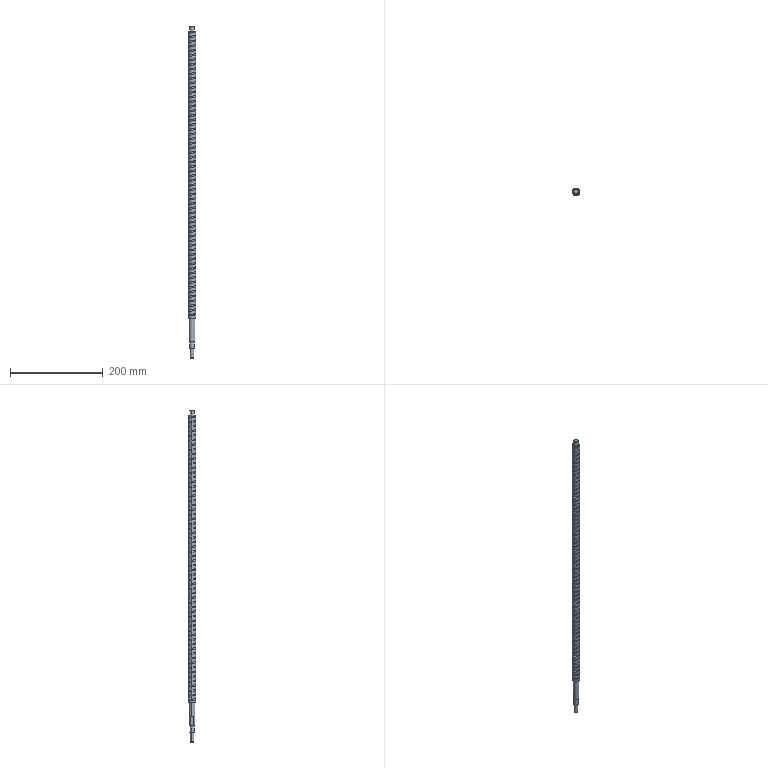Part | STEP file | Handwheel Screw SFUR1605-716 | 1 solid | 164 faces | box 16 x 16 x 716 mm | volume 121693 mm3 | cylinder 138 | plane 16 | cone 9 | spline 1 | commonest cylinder face diameters 16 x126 10 x4 4 x3 8 x2 12 x2 3 x1